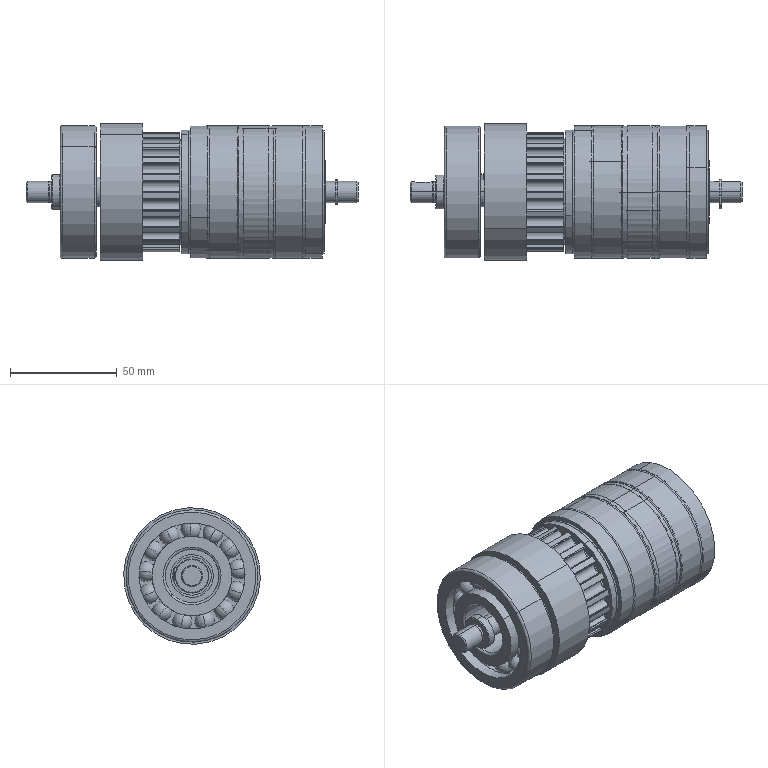Part | SolidWorks | features CompositeCurve 63 | 35 solids | 1559 faces | box 155.5 x 64 x 64 mm | volume 413090 mm3 | cylinder 559 | torus 452 | sphere 234 | plane 193 | spline 82 | cone 39 | commonest cylinder face diameters 0.8 x52 48.125 x41 53.75 x41 5.14 x33 10 x31 2 x20